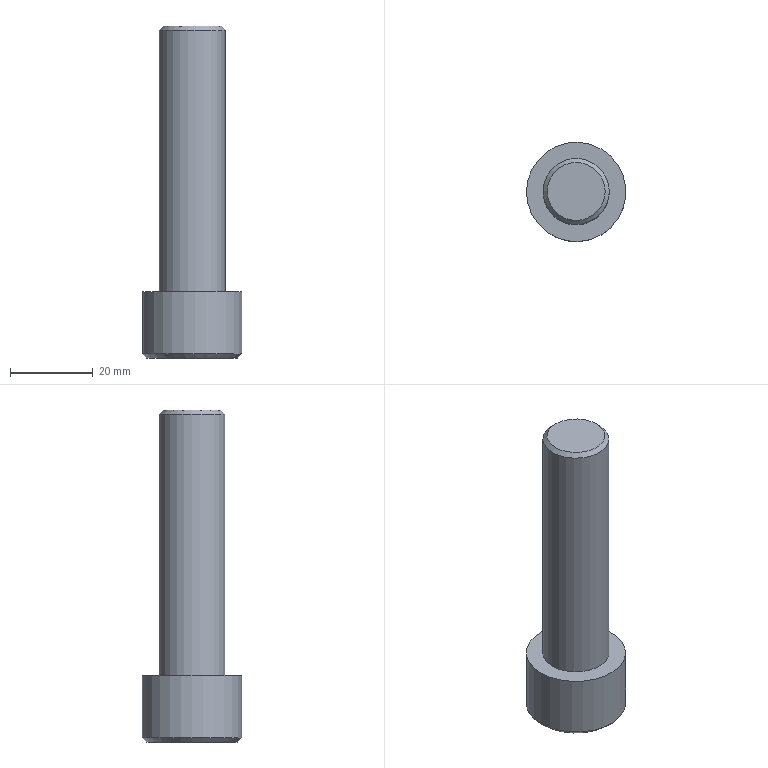Part | STEP file | M16.00-80.00 | 1 solid | 14 faces | box 24 x 24 x 80.203 mm | volume 18728 mm3 | plane 10 | cylinder 2 | cone 2 | commonest cylinder face diameters 16 x1 24 x1